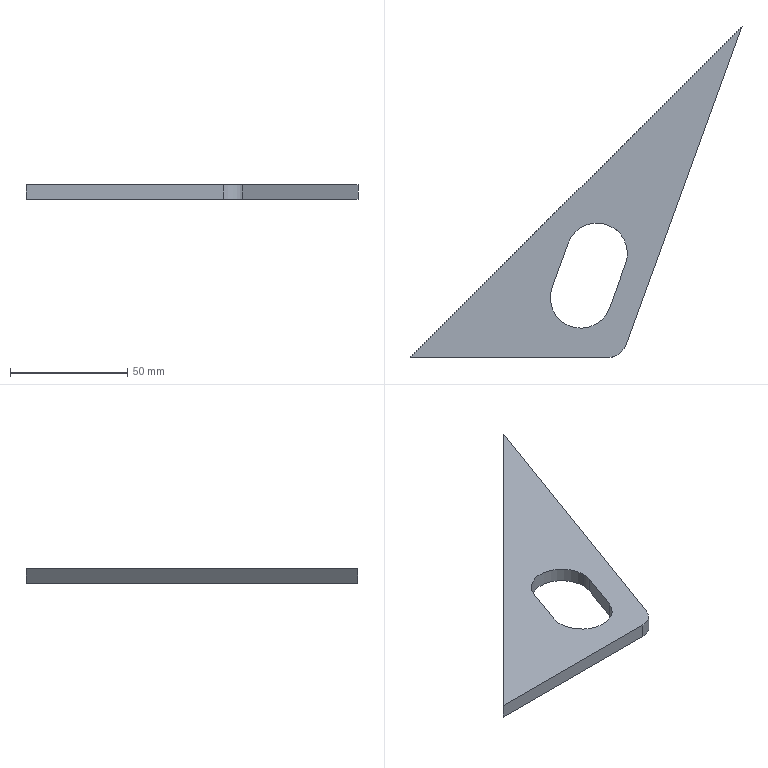Part | SolidWorks | features FlatPattern 1, SMBaseFlange 1, SheetMetal 1 | 1 solid | 11 faces | box 141.303 x 140.954 x 6 mm | volume 31713 mm3 | plane 7 | cylinder 4 | commonest cylinder face diameters 26 x3 17 x1
STEP:
#1=CARTESIAN_POINT('',(92.517,44.294,-6.));
#2=VERTEX_POINT('',#1);
#3=CARTESIAN_POINT('',(67.301,48.74,-6.));
#4=VERTEX_POINT('',#3);
#5=CARTESIAN_POINT('',(79.517,44.294,-6.));
#6=DIRECTION('',(0.,0.,1.));
#7=DIRECTION('',(1.,0.,0.));
#8=AXIS2_PLACEMENT_3D('',#5,#6,#7);
#9=CIRCLE('',#8,13.);
#10=EDGE_CURVE('',#2,#4,#9,.T.);
#11=ORIENTED_EDGE('',*,*,#10,.F.);
#12=CARTESIAN_POINT('',(92.517,44.294,0.));
#13=VERTEX_POINT('',#12);
#14=CARTESIAN_POINT('',(92.517,44.294,-6.));
#15=DIRECTION('',(0.,0.,1.));
#16=VECTOR('',#15,1000.);
#17=LINE('',#14,#16);
#18=EDGE_CURVE('',#2,#13,#17,.T.);
#19=ORIENTED_EDGE('',*,*,#18,.T.);
#20=CARTESIAN_POINT('',(67.301,48.74,0.));
#21=VERTEX_POINT('',#20);
#22=CARTESIAN_POINT('',(79.517,44.294,0.));
#23=DIRECTION('',(0.,0.,1.));
#24=DIRECTION('',(1.,0.,0.));
#25=AXIS2_PLACEMENT_3D('',#22,#23,#24);
#26=CIRCLE('',#25,13.);
#27=EDGE_CURVE('',#13,#21,#26,.T.);
#28=ORIENTED_EDGE('',*,*,#27,.T.);
#29=CARTESIAN_POINT('',(67.301,48.74,-6.));
#30=DIRECTION('',(0.,0.,1.));
#31=VECTOR('',#30,1000.);
#32=LINE('',#29,#31);
#33=EDGE_CURVE('',#4,#21,#32,.T.);
#34=ORIENTED_EDGE('',*,*,#33,.F.);
#35=EDGE_LOOP('',(#11,#19,#28,#34));
#36=FACE_OUTER_BOUND('',#35,.T.);
#37=CARTESIAN_POINT('',(79.517,44.294,-6.));
#38=DIRECTION('',(0.,0.,1.));
#39=DIRECTION('',(1.,0.,0.));
#40=AXIS2_PLACEMENT_3D('',#37,#38,#39);
#41=CYLINDRICAL_SURFACE('',#40,13.);
#42=ADVANCED_FACE('',(#36),#41,.F.);
#43=CARTESIAN_POINT('',(0.,0.,0.));
#44=VERTEX_POINT('',#43);
#45=CARTESIAN_POINT('',(84.048,0.,0.));
#46=VERTEX_POINT('',#45);
#47=CARTESIAN_POINT('',(84.048,0.,0.));
#48=DIRECTION('',(1.,0.,0.));
#49=VECTOR('',#48,1000.);
#50=LINE('',#47,#49);
#51=EDGE_CURVE('',#44,#46,#50,.T.);
#52=ORIENTED_EDGE('',*,*,#51,.F.);
#53=CARTESIAN_POINT('',(0.,0.,-6.));
#54=VERTEX_POINT('',#53);
#55=CARTESIAN_POINT('',(0.,0.,-6.));
#56=DIRECTION('',(0.,0.,1.));
#57=VECTOR('',#56,1000.);
#58=LINE('',#55,#57);
#59=EDGE_CURVE('',#54,#44,#58,.T.);
#60=ORIENTED_EDGE('',*,*,#59,.F.);
#61=CARTESIAN_POINT('',(84.048,0.,-6.));
#62=VERTEX_POINT('',#61);
#63=CARTESIAN_POINT('',(84.048,0.,-6.));
#64=DIRECTION('',(1.,0.,0.));
#65=VECTOR('',#64,1000.);
#66=LINE('',#63,#65);
#67=EDGE_CURVE('',#54,#62,#66,.T.);
#68=ORIENTED_EDGE('',*,*,#67,.T.);
#69=CARTESIAN_POINT('',(84.048,0.,-6.));
#70=DIRECTION('',(0.,0.,1.));
#71=VECTOR('',#70,1000.);
#72=LINE('',#69,#71);
#73=EDGE_CURVE('',#62,#46,#72,.T.);
#74=ORIENTED_EDGE('',*,*,#73,.T.);
#75=EDGE_LOOP('',(#52,#60,#68,#74));
#76=FACE_OUTER_BOUND('',#75,.T.);
#77=CARTESIAN_POINT('',(84.048,0.,-6.));
#78=DIRECTION('',(0.,-1.,0.));
#79=DIRECTION('',(0.,0.,-1.));
#80=AXIS2_PLACEMENT_3D('',#77,#78,#79);
#81=PLANE('',#80);
#82=ADVANCED_FACE('',(#76),#81,.T.);
#83=CARTESIAN_POINT('',(141.303,140.954,0.));
#84=VERTEX_POINT('',#83);
#85=CARTESIAN_POINT('',(0.,0.,0.));
#86=DIRECTION('',(-0.708,-0.7062,0.));
#87=VECTOR('',#86,1000.);
#88=LINE('',#85,#87);
#89=EDGE_CURVE('',#84,#44,#88,.T.);
#90=ORIENTED_EDGE('',*,*,#89,.F.);
#91=CARTESIAN_POINT('',(141.303,140.954,-6.));
#92=VERTEX_POINT('',#91);
#93=CARTESIAN_POINT('',(141.303,140.954,-6.));
#94=DIRECTION('',(0.,0.,1.));
#95=VECTOR('',#94,1000.);
#96=LINE('',#93,#95);
#97=EDGE_CURVE('',#92,#84,#96,.T.);
#98=ORIENTED_EDGE('',*,*,#97,.F.);
#99=CARTESIAN_POINT('',(0.,0.,-6.));
#100=DIRECTION('',(-0.708,-0.7062,0.));
#101=VECTOR('',#100,1000.);
#102=LINE('',#99,#101);
#103=EDGE_CURVE('',#92,#54,#102,.T.);
#104=ORIENTED_EDGE('',*,*,#103,.T.);
#105=ORIENTED_EDGE('',*,*,#59,.T.);
#106=EDGE_LOOP('',(#90,#98,#104,#105));
#107=FACE_OUTER_BOUND('',#106,.T.);
#108=CARTESIAN_POINT('',(0.,0.,-6.));
#109=DIRECTION('',(-0.7062,0.708,0.));
#110=DIRECTION('',(-0.708,-0.7062,0.));
#111=AXIS2_PLACEMENT_3D('',#108,#109,#110);
#112=PLANE('',#111);
#113=ADVANCED_FACE('',(#107),#112,.T.);
#114=CARTESIAN_POINT('',(92.036,5.593,0.));
#115=VERTEX_POINT('',#114);
#116=CARTESIAN_POINT('',(141.303,140.954,0.));
#117=DIRECTION('',(0.342,0.9397,0.));
#118=VECTOR('',#117,1000.);
#119=LINE('',#116,#118);
#120=EDGE_CURVE('',#115,#84,#119,.T.);
#121=ORIENTED_EDGE('',*,*,#120,.F.);
#122=CARTESIAN_POINT('',(92.036,5.593,-6.));
#123=VERTEX_POINT('',#122);
#124=CARTESIAN_POINT('',(92.036,5.593,-6.));
#125=DIRECTION('',(0.,0.,1.));
#126=VECTOR('',#125,1000.);
#127=LINE('',#124,#126);
#128=EDGE_CURVE('',#123,#115,#127,.T.);
#129=ORIENTED_EDGE('',*,*,#128,.F.);
#130=CARTESIAN_POINT('',(141.303,140.954,-6.));
#131=DIRECTION('',(0.342,0.9397,0.));
#132=VECTOR('',#131,1000.);
#133=LINE('',#130,#132);
#134=EDGE_CURVE('',#123,#92,#133,.T.);
#135=ORIENTED_EDGE('',*,*,#134,.T.);
#136=ORIENTED_EDGE('',*,*,#97,.T.);
#137=EDGE_LOOP('',(#121,#129,#135,#136));
#138=FACE_OUTER_BOUND('',#137,.T.);
#139=CARTESIAN_POINT('',(141.303,140.954,-6.));
#140=DIRECTION('',(0.9397,-0.342,0.));
#141=DIRECTION('',(0.342,0.9397,0.));
#142=AXIS2_PLACEMENT_3D('',#139,#140,#141);
#143=PLANE('',#142);
#144=ADVANCED_FACE('',(#138),#143,.T.);
#145=CARTESIAN_POINT('',(84.048,8.5,0.));
#146=DIRECTION('',(0.,0.,1.));
#147=DIRECTION('',(-1.,0.,0.));
#148=AXIS2_PLACEMENT_3D('',#145,#146,#147);
#149=CIRCLE('',#148,8.5);
#150=EDGE_CURVE('',#46,#115,#149,.T.);
#151=ORIENTED_EDGE('',*,*,#150,.F.);
#152=ORIENTED_EDGE('',*,*,#73,.F.);
#153=CARTESIAN_POINT('',(84.048,8.5,-6.));
#154=DIRECTION('',(0.,0.,1.));
#155=DIRECTION('',(-1.,0.,0.));
#156=AXIS2_PLACEMENT_3D('',#153,#154,#155);
#157=CIRCLE('',#156,8.5);
#158=EDGE_CURVE('',#62,#123,#157,.T.);
#159=ORIENTED_EDGE('',*,*,#158,.T.);
#160=ORIENTED_EDGE('',*,*,#128,.T.);
#161=EDGE_LOOP('',(#151,#152,#159,#160));
#162=FACE_OUTER_BOUND('',#161,.T.);
#163=CARTESIAN_POINT('',(84.048,8.5,-6.));
#164=DIRECTION('',(0.,0.,1.));
#165=DIRECTION('',(1.,0.,0.));
#166=AXIS2_PLACEMENT_3D('',#163,#164,#165);
#167=CYLINDRICAL_SURFACE('',#166,8.5);
#168=ADVANCED_FACE('',(#162),#167,.T.);
#169=CARTESIAN_POINT('',(60.461,29.946,-6.));
#170=VERTEX_POINT('',#169);
#171=CARTESIAN_POINT('',(84.893,21.054,-6.));
#172=VERTEX_POINT('',#171);
#173=CARTESIAN_POINT('',(72.677,25.5,-6.));
#174=DIRECTION('',(0.,0.,1.));
#175=DIRECTION('',(1.,0.,0.));
#176=AXIS2_PLACEMENT_3D('',#173,#174,#175);
#177=CIRCLE('',#176,13.);
#178=EDGE_CURVE('',#170,#172,#177,.T.);
#179=ORIENTED_EDGE('',*,*,#178,.T.);
#180=CARTESIAN_POINT('',(91.733,39.848,-6.));
#181=VERTEX_POINT('',#180);
#182=CARTESIAN_POINT('',(84.893,21.054,-6.));
#183=DIRECTION('',(0.342,0.9397,0.));
#184=VECTOR('',#183,1000.);
#185=LINE('',#182,#184);
#186=EDGE_CURVE('',#172,#181,#185,.T.);
#187=ORIENTED_EDGE('',*,*,#186,.T.);
#188=CARTESIAN_POINT('',(79.517,44.294,-6.));
#189=DIRECTION('',(0.,0.,1.));
#190=DIRECTION('',(1.,0.,0.));
#191=AXIS2_PLACEMENT_3D('',#188,#189,#190);
#192=CIRCLE('',#191,13.);
#193=EDGE_CURVE('',#181,#2,#192,.T.);
#194=ORIENTED_EDGE('',*,*,#193,.T.);
#195=ORIENTED_EDGE('',*,*,#10,.T.);
#196=CARTESIAN_POINT('',(60.461,29.946,-6.));
#197=DIRECTION('',(-0.342,-0.9397,0.));
#198=VECTOR('',#197,1000.);
#199=LINE('',#196,#198);
#200=EDGE_CURVE('',#4,#170,#199,.T.);
#201=ORIENTED_EDGE('',*,*,#200,.T.);
#202=EDGE_LOOP('',(#179,#187,#194,#195,#201));
#203=FACE_BOUND('',#202,.T.);
#204=ORIENTED_EDGE('',*,*,#67,.F.);
#205=ORIENTED_EDGE('',*,*,#103,.F.);
#206=ORIENTED_EDGE('',*,*,#134,.F.);
#207=ORIENTED_EDGE('',*,*,#158,.F.);
#208=EDGE_LOOP('',(#204,#205,#206,#207));
#209=FACE_OUTER_BOUND('',#208,.T.);
#210=CARTESIAN_POINT('',(84.048,8.5,-6.));
#211=DIRECTION('',(0.,0.,-1.));
#212=DIRECTION('',(-1.,0.,0.));
#213=AXIS2_PLACEMENT_3D('',#210,#211,#212);
#214=PLANE('',#213);
#215=ADVANCED_FACE('',(#203,#209),#214,.T.);
#216=CARTESIAN_POINT('',(84.893,21.054,0.));
#217=VERTEX_POINT('',#216);
#218=CARTESIAN_POINT('',(91.733,39.848,0.));
#219=VERTEX_POINT('',#218);
#220=CARTESIAN_POINT('',(84.893,21.054,0.));
#221=DIRECTION('',(0.342,0.9397,0.));
#222=VECTOR('',#221,1000.);
#223=LINE('',#220,#222);
#224=EDGE_CURVE('',#217,#219,#223,.T.);
#225=ORIENTED_EDGE('',*,*,#224,.F.);
#226=CARTESIAN_POINT('',(60.461,29.946,0.));
#227=VERTEX_POINT('',#226);
#228=CARTESIAN_POINT('',(72.677,25.5,0.));
#229=DIRECTION('',(0.,0.,1.));
#230=DIRECTION('',(1.,0.,0.));
#231=AXIS2_PLACEMENT_3D('',#228,#229,#230);
#232=CIRCLE('',#231,13.);
#233=EDGE_CURVE('',#227,#217,#232,.T.);
#234=ORIENTED_EDGE('',*,*,#233,.F.);
#235=CARTESIAN_POINT('',(60.461,29.946,0.));
#236=DIRECTION('',(-0.342,-0.9397,0.));
#237=VECTOR('',#236,1000.);
#238=LINE('',#235,#237);
#239=EDGE_CURVE('',#21,#227,#238,.T.);
#240=ORIENTED_EDGE('',*,*,#239,.F.);
#241=ORIENTED_EDGE('',*,*,#27,.F.);
#242=CARTESIAN_POINT('',(79.517,44.294,0.));
#243=DIRECTION('',(0.,0.,1.));
#244=DIRECTION('',(1.,0.,0.));
#245=AXIS2_PLACEMENT_3D('',#242,#243,#244);
#246=CIRCLE('',#245,13.);
#247=EDGE_CURVE('',#219,#13,#246,.T.);
#248=ORIENTED_EDGE('',*,*,#247,.F.);
#249=EDGE_LOOP('',(#225,#234,#240,#241,#248));
#250=FACE_BOUND('',#249,.T.);
#251=ORIENTED_EDGE('',*,*,#51,.T.);
#252=ORIENTED_EDGE('',*,*,#150,.T.);
#253=ORIENTED_EDGE('',*,*,#120,.T.);
#254=ORIENTED_EDGE('',*,*,#89,.T.);
#255=EDGE_LOOP('',(#251,#252,#253,#254));
#256=FACE_OUTER_BOUND('',#255,.T.);
#257=CARTESIAN_POINT('',(84.048,8.5,0.));
#258=DIRECTION('',(0.,0.,-1.));
#259=DIRECTION('',(-1.,0.,0.));
#260=AXIS2_PLACEMENT_3D('',#257,#258,#259);
#261=PLANE('',#260);
#262=ADVANCED_FACE('',(#250,#256),#261,.F.);
#263=ORIENTED_EDGE('',*,*,#233,.T.);
#264=CARTESIAN_POINT('',(84.893,21.054,-6.));
#265=DIRECTION('',(0.,0.,1.));
#266=VECTOR('',#265,1000.);
#267=LINE('',#264,#266);
#268=EDGE_CURVE('',#172,#217,#267,.T.);
#269=ORIENTED_EDGE('',*,*,#268,.F.);
#270=ORIENTED_EDGE('',*,*,#178,.F.);
#271=CARTESIAN_POINT('',(60.461,29.946,-6.));
#272=DIRECTION('',(0.,0.,1.));
#273=VECTOR('',#272,1000.);
#274=LINE('',#271,#273);
#275=EDGE_CURVE('',#170,#227,#274,.T.);
#276=ORIENTED_EDGE('',*,*,#275,.T.);
#277=EDGE_LOOP('',(#263,#269,#270,#276));
#278=FACE_OUTER_BOUND('',#277,.T.);
#279=CARTESIAN_POINT('',(72.677,25.5,-6.));
#280=DIRECTION('',(0.,0.,1.));
#281=DIRECTION('',(1.,0.,0.));
#282=AXIS2_PLACEMENT_3D('',#279,#280,#281);
#283=CYLINDRICAL_SURFACE('',#282,13.);
#284=ADVANCED_FACE('',(#278),#283,.F.);
#285=ORIENTED_EDGE('',*,*,#239,.T.);
#286=ORIENTED_EDGE('',*,*,#275,.F.);
#287=ORIENTED_EDGE('',*,*,#200,.F.);
#288=ORIENTED_EDGE('',*,*,#33,.T.);
#289=EDGE_LOOP('',(#285,#286,#287,#288));
#290=FACE_OUTER_BOUND('',#289,.T.);
#291=CARTESIAN_POINT('',(60.461,29.946,-6.));
#292=DIRECTION('',(-0.9397,0.342,0.));
#293=DIRECTION('',(-0.342,-0.9397,0.));
#294=AXIS2_PLACEMENT_3D('',#291,#292,#293);
#295=PLANE('',#294);
#296=ADVANCED_FACE('',(#290),#295,.F.);
#297=ORIENTED_EDGE('',*,*,#18,.F.);
#298=ORIENTED_EDGE('',*,*,#193,.F.);
#299=CARTESIAN_POINT('',(91.733,39.848,-6.));
#300=DIRECTION('',(0.,0.,1.));
#301=VECTOR('',#300,1000.);
#302=LINE('',#299,#301);
#303=EDGE_CURVE('',#181,#219,#302,.T.);
#304=ORIENTED_EDGE('',*,*,#303,.T.);
#305=ORIENTED_EDGE('',*,*,#247,.T.);
#306=EDGE_LOOP('',(#297,#298,#304,#305));
#307=FACE_OUTER_BOUND('',#306,.T.);
#308=CARTESIAN_POINT('',(79.517,44.294,-6.));
#309=DIRECTION('',(0.,0.,1.));
#310=DIRECTION('',(1.,0.,0.));
#311=AXIS2_PLACEMENT_3D('',#308,#309,#310);
#312=CYLINDRICAL_SURFACE('',#311,13.);
#313=ADVANCED_FACE('',(#307),#312,.F.);
#314=ORIENTED_EDGE('',*,*,#224,.T.);
#315=ORIENTED_EDGE('',*,*,#303,.F.);
#316=ORIENTED_EDGE('',*,*,#186,.F.);
#317=ORIENTED_EDGE('',*,*,#268,.T.);
#318=EDGE_LOOP('',(#314,#315,#316,#317));
#319=FACE_OUTER_BOUND('',#318,.T.);
#320=CARTESIAN_POINT('',(84.893,21.054,-6.));
#321=DIRECTION('',(0.9397,-0.342,0.));
#322=DIRECTION('',(0.342,0.9397,0.));
#323=AXIS2_PLACEMENT_3D('',#320,#321,#322);
#324=PLANE('',#323);
#325=ADVANCED_FACE('',(#319),#324,.F.);
#326=CLOSED_SHELL('',(#42,#82,#113,#144,#168,#215,#262,#284,#296,#313,#325));
#327=MANIFOLD_SOLID_BREP('',#326);
#328=CARTESIAN_POINT('',(0.,0.,0.));
#329=DIRECTION('',(0.,0.,1.));
#330=DIRECTION('',(1.,0.,0.));
#331=AXIS2_PLACEMENT_3D('',#328,#329,#330);
#332=(LENGTH_UNIT()NAMED_UNIT(*)SI_UNIT(.MILLI.,.METRE.));
#333=UNCERTAINTY_MEASURE_WITH_UNIT(LENGTH_MEASURE(0.00001),#332,'','');
#334=(NAMED_UNIT(*)PLANE_ANGLE_UNIT()SI_UNIT($,.RADIAN.));
#335=(NAMED_UNIT(*)SI_UNIT($,.STERADIAN.)SOLID_ANGLE_UNIT());
#336=(GEOMETRIC_REPRESENTATION_CONTEXT(3)GLOBAL_UNCERTAINTY_ASSIGNED_CONTEXT((#333))GLOBAL_UNIT_ASSIGNED_CONTEXT((#332,#334,#335))REPRESENTATION_CONTEXT('',''));
#337=ADVANCED_BREP_SHAPE_REPRESENTATION('',(#327,#331),#336);